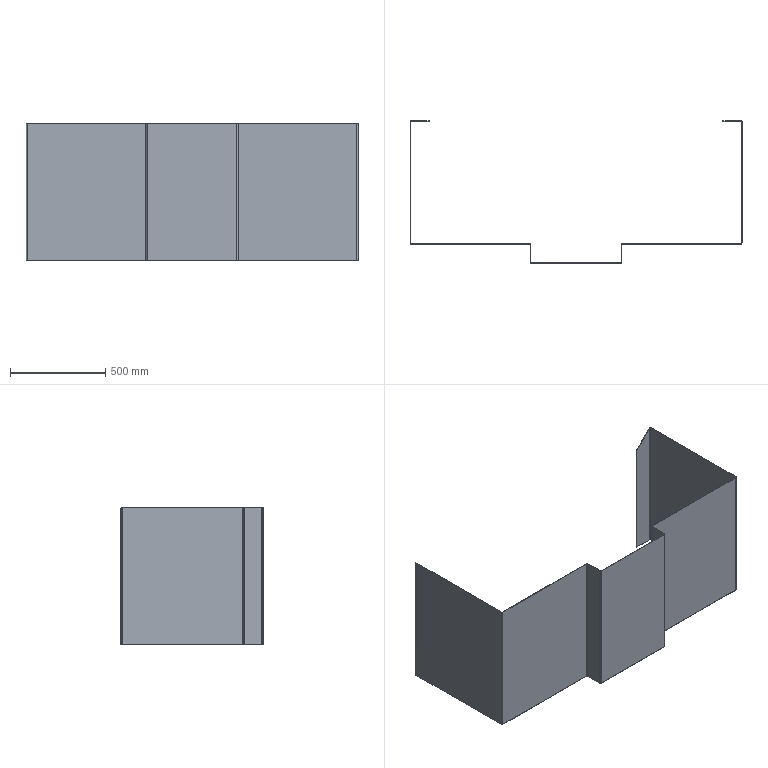Part | STEP file | Double-tube frame cover plate SGN-1-01 | 1 solid | 70 faces | box 1740 x 745 x 720 mm | volume 7319449 mm3 | plane 54 | cylinder 16 | commonest cylinder face diameters 6 x8 12 x8